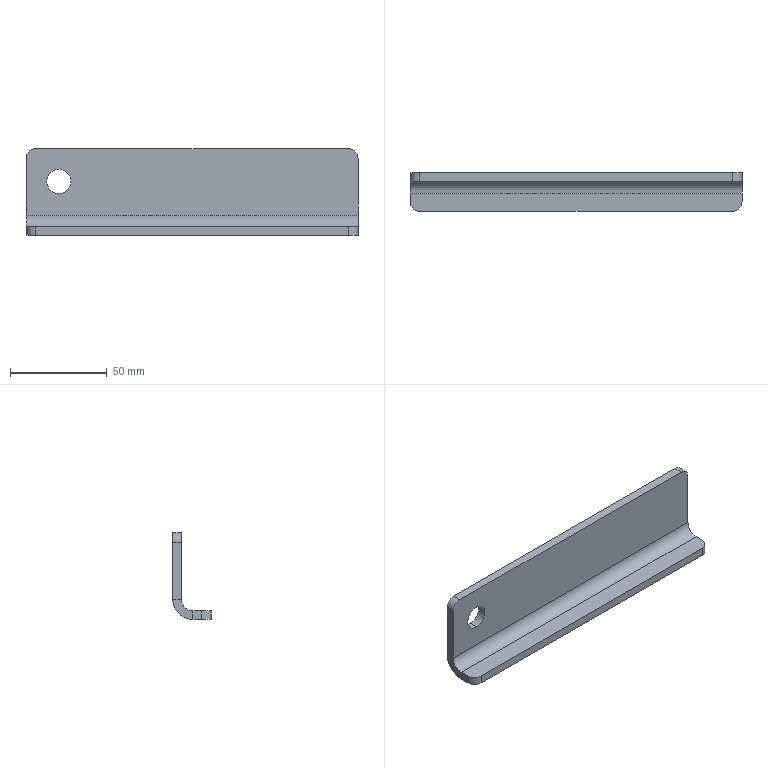Part | SolidWorks | features Fillet 1, FlatPattern 1, ICE 1, SMBaseFlange 1, SheetMetal 1 | 1 solid | 20 faces | box 172 x 20 x 45 mm | volume 43438 mm3 | plane 12 | cylinder 8 | commonest cylinder face diameters 10 x4 12.5 x2 12 x1 21 x1
STEP:
#1=CARTESIAN_POINT('',(17.,15.5,21.75));
#2=VERTEX_POINT('',#1);
#3=CARTESIAN_POINT('',(17.,15.5,34.25));
#4=VERTEX_POINT('',#3);
#5=CARTESIAN_POINT('',(17.,15.5,28.));
#6=DIRECTION('',(0.,1.,0.));
#7=DIRECTION('',(0.,0.,-1.));
#8=AXIS2_PLACEMENT_3D('',#5,#6,#7);
#9=CIRCLE('',#8,6.25);
#10=EDGE_CURVE('',#2,#4,#9,.T.);
#11=ORIENTED_EDGE('',*,*,#10,.F.);
#12=CARTESIAN_POINT('',(17.,20.,21.75));
#13=VERTEX_POINT('',#12);
#14=CARTESIAN_POINT('',(17.,-0.001,21.75));
#15=DIRECTION('',(0.,1.,0.));
#16=VECTOR('',#15,1000.);
#17=LINE('',#14,#16);
#18=EDGE_CURVE('',#2,#13,#17,.T.);
#19=ORIENTED_EDGE('',*,*,#18,.T.);
#20=CARTESIAN_POINT('',(17.,20.,34.25));
#21=VERTEX_POINT('',#20);
#22=CARTESIAN_POINT('',(17.,20.,28.));
#23=DIRECTION('',(0.,1.,0.));
#24=DIRECTION('',(0.,0.,1.));
#25=AXIS2_PLACEMENT_3D('',#22,#23,#24);
#26=CIRCLE('',#25,6.25);
#27=EDGE_CURVE('',#13,#21,#26,.T.);
#28=ORIENTED_EDGE('',*,*,#27,.T.);
#29=CARTESIAN_POINT('',(17.,-0.001,34.25));
#30=DIRECTION('',(0.,1.,0.));
#31=VECTOR('',#30,1000.);
#32=LINE('',#29,#31);
#33=EDGE_CURVE('',#4,#21,#32,.T.);
#34=ORIENTED_EDGE('',*,*,#33,.F.);
#35=EDGE_LOOP('',(#11,#19,#28,#34));
#36=FACE_OUTER_BOUND('',#35,.T.);
#37=CARTESIAN_POINT('',(17.,-0.001,28.));
#38=DIRECTION('',(0.,1.,0.));
#39=DIRECTION('',(0.,0.,1.));
#40=AXIS2_PLACEMENT_3D('',#37,#38,#39);
#41=CYLINDRICAL_SURFACE('',#40,6.25);
#42=ADVANCED_FACE('',(#36),#41,.F.);
#43=CARTESIAN_POINT('',(172.,9.5,0.));
#44=VERTEX_POINT('',#43);
#45=CARTESIAN_POINT('',(172.,9.5,4.5));
#46=VERTEX_POINT('',#45);
#47=CARTESIAN_POINT('',(172.,9.5,0.));
#48=DIRECTION('',(0.,0.,1.));
#49=VECTOR('',#48,1000.);
#50=LINE('',#47,#49);
#51=EDGE_CURVE('',#44,#46,#50,.T.);
#52=ORIENTED_EDGE('',*,*,#51,.F.);
#53=CARTESIAN_POINT('',(172.,20.,10.5));
#54=VERTEX_POINT('',#53);
#55=CARTESIAN_POINT('',(172.,9.5,10.5));
#56=DIRECTION('',(1.,0.,0.));
#57=DIRECTION('',(0.,0.,1.));
#58=AXIS2_PLACEMENT_3D('',#55,#56,#57);
#59=CIRCLE('',#58,10.5);
#60=EDGE_CURVE('',#44,#54,#59,.T.);
#61=ORIENTED_EDGE('',*,*,#60,.T.);
#62=CARTESIAN_POINT('',(172.,15.5,10.5));
#63=VERTEX_POINT('',#62);
#64=CARTESIAN_POINT('',(172.,15.5,10.5));
#65=DIRECTION('',(0.,1.,0.));
#66=VECTOR('',#65,1000.);
#67=LINE('',#64,#66);
#68=EDGE_CURVE('',#63,#54,#67,.T.);
#69=ORIENTED_EDGE('',*,*,#68,.F.);
#70=CARTESIAN_POINT('',(172.,9.5,10.5));
#71=DIRECTION('',(1.,0.,0.));
#72=DIRECTION('',(0.,0.,-1.));
#73=AXIS2_PLACEMENT_3D('',#70,#71,#72);
#74=CIRCLE('',#73,6.);
#75=EDGE_CURVE('',#46,#63,#74,.T.);
#76=ORIENTED_EDGE('',*,*,#75,.F.);
#77=EDGE_LOOP('',(#52,#61,#69,#76));
#78=FACE_OUTER_BOUND('',#77,.T.);
#79=CARTESIAN_POINT('',(172.,9.5,0.));
#80=DIRECTION('',(1.,0.,0.));
#81=DIRECTION('',(0.,0.,-1.));
#82=AXIS2_PLACEMENT_3D('',#79,#80,#81);
#83=PLANE('',#82);
#84=ADVANCED_FACE('',(#78),#83,.T.);
#85=CARTESIAN_POINT('',(172.,5.,4.5));
#86=VERTEX_POINT('',#85);
#87=CARTESIAN_POINT('',(172.,0.,4.5));
#88=DIRECTION('',(0.,1.,0.));
#89=VECTOR('',#88,1000.);
#90=LINE('',#87,#89);
#91=EDGE_CURVE('',#86,#46,#90,.T.);
#92=ORIENTED_EDGE('',*,*,#91,.F.);
#93=CARTESIAN_POINT('',(172.,5.,0.));
#94=VERTEX_POINT('',#93);
#95=CARTESIAN_POINT('',(172.,5.,10.5));
#96=DIRECTION('',(0.,0.,-1.));
#97=VECTOR('',#96,1000.);
#98=LINE('',#95,#97);
#99=EDGE_CURVE('',#86,#94,#98,.T.);
#100=ORIENTED_EDGE('',*,*,#99,.T.);
#101=CARTESIAN_POINT('',(172.,0.,0.));
#102=DIRECTION('',(0.,1.,0.));
#103=VECTOR('',#102,1000.);
#104=LINE('',#101,#103);
#105=EDGE_CURVE('',#94,#44,#104,.T.);
#106=ORIENTED_EDGE('',*,*,#105,.T.);
#107=ORIENTED_EDGE('',*,*,#51,.T.);
#108=EDGE_LOOP('',(#92,#100,#106,#107));
#109=FACE_OUTER_BOUND('',#108,.T.);
#110=CARTESIAN_POINT('',(172.,15.5,10.5));
#111=DIRECTION('',(1.,0.,0.));
#112=DIRECTION('',(0.,0.,-1.));
#113=AXIS2_PLACEMENT_3D('',#110,#111,#112);
#114=PLANE('',#113);
#115=ADVANCED_FACE('',(#109),#114,.T.);
#116=CARTESIAN_POINT('',(0.,20.,10.5));
#117=VERTEX_POINT('',#116);
#118=CARTESIAN_POINT('',(0.,15.5,10.5));
#119=VERTEX_POINT('',#118);
#120=CARTESIAN_POINT('',(0.,20.,10.5));
#121=DIRECTION('',(0.,-1.,0.));
#122=VECTOR('',#121,1000.);
#123=LINE('',#120,#122);
#124=EDGE_CURVE('',#117,#119,#123,.T.);
#125=ORIENTED_EDGE('',*,*,#124,.F.);
#126=CARTESIAN_POINT('',(0.,9.5,0.));
#127=VERTEX_POINT('',#126);
#128=CARTESIAN_POINT('',(0.,9.5,10.5));
#129=DIRECTION('',(1.,0.,0.));
#130=DIRECTION('',(0.,0.,1.));
#131=AXIS2_PLACEMENT_3D('',#128,#129,#130);
#132=CIRCLE('',#131,10.5);
#133=EDGE_CURVE('',#127,#117,#132,.T.);
#134=ORIENTED_EDGE('',*,*,#133,.F.);
#135=CARTESIAN_POINT('',(0.,9.5,4.5));
#136=VERTEX_POINT('',#135);
#137=CARTESIAN_POINT('',(0.,9.5,4.5));
#138=DIRECTION('',(0.,0.,-1.));
#139=VECTOR('',#138,1000.);
#140=LINE('',#137,#139);
#141=EDGE_CURVE('',#136,#127,#140,.T.);
#142=ORIENTED_EDGE('',*,*,#141,.F.);
#143=CARTESIAN_POINT('',(0.,9.5,10.5));
#144=DIRECTION('',(1.,0.,0.));
#145=DIRECTION('',(0.,0.,-1.));
#146=AXIS2_PLACEMENT_3D('',#143,#144,#145);
#147=CIRCLE('',#146,6.);
#148=EDGE_CURVE('',#136,#119,#147,.T.);
#149=ORIENTED_EDGE('',*,*,#148,.T.);
#150=EDGE_LOOP('',(#125,#134,#142,#149));
#151=FACE_OUTER_BOUND('',#150,.T.);
#152=CARTESIAN_POINT('',(0.,20.,10.5));
#153=DIRECTION('',(-1.,0.,0.));
#154=DIRECTION('',(0.,0.,1.));
#155=AXIS2_PLACEMENT_3D('',#152,#153,#154);
#156=PLANE('',#155);
#157=ADVANCED_FACE('',(#151),#156,.T.);
#158=CARTESIAN_POINT('',(0.,15.5,40.));
#159=VERTEX_POINT('',#158);
#160=CARTESIAN_POINT('',(0.,15.5,0.));
#161=DIRECTION('',(0.,0.,1.));
#162=VECTOR('',#161,1000.);
#163=LINE('',#160,#162);
#164=EDGE_CURVE('',#119,#159,#163,.T.);
#165=ORIENTED_EDGE('',*,*,#164,.T.);
#166=CARTESIAN_POINT('',(0.,20.,40.));
#167=VERTEX_POINT('',#166);
#168=CARTESIAN_POINT('',(0.,9.5,40.));
#169=DIRECTION('',(0.,1.,0.));
#170=VECTOR('',#169,1000.);
#171=LINE('',#168,#170);
#172=EDGE_CURVE('',#159,#167,#171,.T.);
#173=ORIENTED_EDGE('',*,*,#172,.T.);
#174=CARTESIAN_POINT('',(0.,20.,0.));
#175=DIRECTION('',(0.,0.,1.));
#176=VECTOR('',#175,1000.);
#177=LINE('',#174,#176);
#178=EDGE_CURVE('',#117,#167,#177,.T.);
#179=ORIENTED_EDGE('',*,*,#178,.F.);
#180=ORIENTED_EDGE('',*,*,#124,.T.);
#181=EDGE_LOOP('',(#165,#173,#179,#180));
#182=FACE_OUTER_BOUND('',#181,.T.);
#183=CARTESIAN_POINT('',(0.,9.5,4.5));
#184=DIRECTION('',(-1.,0.,0.));
#185=DIRECTION('',(0.,0.,1.));
#186=AXIS2_PLACEMENT_3D('',#183,#184,#185);
#187=PLANE('',#186);
#188=ADVANCED_FACE('',(#182),#187,.T.);
#189=CARTESIAN_POINT('',(17.,20.,28.));
#190=DIRECTION('',(0.,1.,0.));
#191=DIRECTION('',(0.,0.,1.));
#192=AXIS2_PLACEMENT_3D('',#189,#190,#191);
#193=CIRCLE('',#192,6.25);
#194=EDGE_CURVE('',#21,#13,#193,.T.);
#195=ORIENTED_EDGE('',*,*,#194,.F.);
#196=ORIENTED_EDGE('',*,*,#27,.F.);
#197=EDGE_LOOP('',(#195,#196));
#198=FACE_BOUND('',#197,.T.);
#199=CARTESIAN_POINT('',(167.,20.,45.));
#200=VERTEX_POINT('',#199);
#201=CARTESIAN_POINT('',(5.,20.,45.));
#202=VERTEX_POINT('',#201);
#203=CARTESIAN_POINT('',(172.,20.,45.));
#204=DIRECTION('',(-1.,0.,0.));
#205=VECTOR('',#204,1000.);
#206=LINE('',#203,#205);
#207=EDGE_CURVE('',#200,#202,#206,.T.);
#208=ORIENTED_EDGE('',*,*,#207,.F.);
#209=CARTESIAN_POINT('',(172.,20.,40.));
#210=VERTEX_POINT('',#209);
#211=CARTESIAN_POINT('',(167.,20.,40.));
#212=DIRECTION('',(0.,1.,0.));
#213=DIRECTION('',(0.,0.,-1.));
#214=AXIS2_PLACEMENT_3D('',#211,#212,#213);
#215=CIRCLE('',#214,5.);
#216=EDGE_CURVE('',#200,#210,#215,.T.);
#217=ORIENTED_EDGE('',*,*,#216,.T.);
#218=CARTESIAN_POINT('',(172.,20.,0.));
#219=DIRECTION('',(0.,0.,1.));
#220=VECTOR('',#219,1000.);
#221=LINE('',#218,#220);
#222=EDGE_CURVE('',#54,#210,#221,.T.);
#223=ORIENTED_EDGE('',*,*,#222,.F.);
#224=CARTESIAN_POINT('',(172.,20.,10.5));
#225=DIRECTION('',(-1.,0.,0.));
#226=VECTOR('',#225,1000.);
#227=LINE('',#224,#226);
#228=EDGE_CURVE('',#54,#117,#227,.T.);
#229=ORIENTED_EDGE('',*,*,#228,.T.);
#230=ORIENTED_EDGE('',*,*,#178,.T.);
#231=CARTESIAN_POINT('',(5.,20.,40.));
#232=DIRECTION('',(0.,1.,0.));
#233=DIRECTION('',(0.,0.,-1.));
#234=AXIS2_PLACEMENT_3D('',#231,#232,#233);
#235=CIRCLE('',#234,5.);
#236=EDGE_CURVE('',#167,#202,#235,.T.);
#237=ORIENTED_EDGE('',*,*,#236,.T.);
#238=EDGE_LOOP('',(#208,#217,#223,#229,#230,#237));
#239=FACE_OUTER_BOUND('',#238,.T.);
#240=CARTESIAN_POINT('',(172.,20.,0.));
#241=DIRECTION('',(0.,-1.,0.));
#242=DIRECTION('',(0.,0.,-1.));
#243=AXIS2_PLACEMENT_3D('',#240,#241,#242);
#244=PLANE('',#243);
#245=ADVANCED_FACE('',(#198,#239),#244,.F.);
#246=CARTESIAN_POINT('',(167.,15.5,45.));
#247=VERTEX_POINT('',#246);
#248=CARTESIAN_POINT('',(5.,15.5,45.));
#249=VERTEX_POINT('',#248);
#250=CARTESIAN_POINT('',(172.,15.5,45.));
#251=DIRECTION('',(-1.,0.,0.));
#252=VECTOR('',#251,1000.);
#253=LINE('',#250,#252);
#254=EDGE_CURVE('',#247,#249,#253,.T.);
#255=ORIENTED_EDGE('',*,*,#254,.F.);
#256=CARTESIAN_POINT('',(167.,15.5,45.));
#257=DIRECTION('',(0.,1.,0.));
#258=VECTOR('',#257,1000.);
#259=LINE('',#256,#258);
#260=EDGE_CURVE('',#247,#200,#259,.T.);
#261=ORIENTED_EDGE('',*,*,#260,.T.);
#262=ORIENTED_EDGE('',*,*,#207,.T.);
#263=CARTESIAN_POINT('',(5.,15.5,45.));
#264=DIRECTION('',(0.,-1.,0.));
#265=VECTOR('',#264,1000.);
#266=LINE('',#263,#265);
#267=EDGE_CURVE('',#202,#249,#266,.T.);
#268=ORIENTED_EDGE('',*,*,#267,.T.);
#269=EDGE_LOOP('',(#255,#261,#262,#268));
#270=FACE_OUTER_BOUND('',#269,.T.);
#271=CARTESIAN_POINT('',(172.,15.5,45.));
#272=DIRECTION('',(0.,0.,1.));
#273=DIRECTION('',(1.,0.,0.));
#274=AXIS2_PLACEMENT_3D('',#271,#272,#273);
#275=PLANE('',#274);
#276=ADVANCED_FACE('',(#270),#275,.T.);
#277=CARTESIAN_POINT('',(17.,15.5,28.));
#278=DIRECTION('',(0.,1.,0.));
#279=DIRECTION('',(0.,0.,-1.));
#280=AXIS2_PLACEMENT_3D('',#277,#278,#279);
#281=CIRCLE('',#280,6.25);
#282=EDGE_CURVE('',#4,#2,#281,.T.);
#283=ORIENTED_EDGE('',*,*,#282,.T.);
#284=ORIENTED_EDGE('',*,*,#10,.T.);
#285=EDGE_LOOP('',(#283,#284));
#286=FACE_BOUND('',#285,.T.);
#287=CARTESIAN_POINT('',(172.,15.5,40.));
#288=VERTEX_POINT('',#287);
#289=CARTESIAN_POINT('',(172.,15.5,0.));
#290=DIRECTION('',(0.,0.,1.));
#291=VECTOR('',#290,1000.);
#292=LINE('',#289,#291);
#293=EDGE_CURVE('',#63,#288,#292,.T.);
#294=ORIENTED_EDGE('',*,*,#293,.T.);
#295=CARTESIAN_POINT('',(167.,15.5,40.));
#296=DIRECTION('',(0.,-1.,0.));
#297=DIRECTION('',(0.,0.,-1.));
#298=AXIS2_PLACEMENT_3D('',#295,#296,#297);
#299=CIRCLE('',#298,5.);
#300=EDGE_CURVE('',#288,#247,#299,.T.);
#301=ORIENTED_EDGE('',*,*,#300,.T.);
#302=ORIENTED_EDGE('',*,*,#254,.T.);
#303=CARTESIAN_POINT('',(5.,15.5,40.));
#304=DIRECTION('',(0.,-1.,0.));
#305=DIRECTION('',(0.,0.,-1.));
#306=AXIS2_PLACEMENT_3D('',#303,#304,#305);
#307=CIRCLE('',#306,5.);
#308=EDGE_CURVE('',#249,#159,#307,.T.);
#309=ORIENTED_EDGE('',*,*,#308,.T.);
#310=ORIENTED_EDGE('',*,*,#164,.F.);
#311=CARTESIAN_POINT('',(172.,15.5,10.5));
#312=DIRECTION('',(-1.,0.,0.));
#313=VECTOR('',#312,1000.);
#314=LINE('',#311,#313);
#315=EDGE_CURVE('',#63,#119,#314,.T.);
#316=ORIENTED_EDGE('',*,*,#315,.F.);
#317=EDGE_LOOP('',(#294,#301,#302,#309,#310,#316));
#318=FACE_OUTER_BOUND('',#317,.T.);
#319=CARTESIAN_POINT('',(172.,15.5,0.));
#320=DIRECTION('',(0.,-1.,0.));
#321=DIRECTION('',(0.,0.,-1.));
#322=AXIS2_PLACEMENT_3D('',#319,#320,#321);
#323=PLANE('',#322);
#324=ADVANCED_FACE('',(#286,#318),#323,.T.);
#325=ORIENTED_EDGE('',*,*,#148,.F.);
#326=CARTESIAN_POINT('',(172.,9.5,4.5));
#327=DIRECTION('',(-1.,0.,0.));
#328=VECTOR('',#327,1000.);
#329=LINE('',#326,#328);
#330=EDGE_CURVE('',#46,#136,#329,.T.);
#331=ORIENTED_EDGE('',*,*,#330,.F.);
#332=ORIENTED_EDGE('',*,*,#75,.T.);
#333=ORIENTED_EDGE('',*,*,#315,.T.);
#334=EDGE_LOOP('',(#325,#331,#332,#333));
#335=FACE_OUTER_BOUND('',#334,.T.);
#336=CARTESIAN_POINT('',(172.,9.5,10.5));
#337=DIRECTION('',(-1.,0.,0.));
#338=DIRECTION('',(0.,0.,1.));
#339=AXIS2_PLACEMENT_3D('',#336,#337,#338);
#340=CYLINDRICAL_SURFACE('',#339,6.);
#341=ADVANCED_FACE('',(#335),#340,.F.);
#342=CARTESIAN_POINT('',(167.,0.,4.5));
#343=VERTEX_POINT('',#342);
#344=CARTESIAN_POINT('',(5.,0.,4.5));
#345=VERTEX_POINT('',#344);
#346=CARTESIAN_POINT('',(172.,0.,4.5));
#347=DIRECTION('',(-1.,0.,0.));
#348=VECTOR('',#347,1000.);
#349=LINE('',#346,#348);
#350=EDGE_CURVE('',#343,#345,#349,.T.);
#351=ORIENTED_EDGE('',*,*,#350,.F.);
#352=CARTESIAN_POINT('',(167.,5.,4.5));
#353=DIRECTION('',(0.,0.,1.));
#354=DIRECTION('',(1.,0.,0.));
#355=AXIS2_PLACEMENT_3D('',#352,#353,#354);
#356=CIRCLE('',#355,5.);
#357=EDGE_CURVE('',#343,#86,#356,.T.);
#358=ORIENTED_EDGE('',*,*,#357,.T.);
#359=ORIENTED_EDGE('',*,*,#91,.T.);
#360=ORIENTED_EDGE('',*,*,#330,.T.);
#361=CARTESIAN_POINT('',(0.,5.,4.5));
#362=VERTEX_POINT('',#361);
#363=CARTESIAN_POINT('',(0.,0.,4.5));
#364=DIRECTION('',(0.,1.,0.));
#365=VECTOR('',#364,1000.);
#366=LINE('',#363,#365);
#367=EDGE_CURVE('',#362,#136,#366,.T.);
#368=ORIENTED_EDGE('',*,*,#367,.F.);
#369=CARTESIAN_POINT('',(5.,5.,4.5));
#370=DIRECTION('',(0.,0.,1.));
#371=DIRECTION('',(1.,0.,0.));
#372=AXIS2_PLACEMENT_3D('',#369,#370,#371);
#373=CIRCLE('',#372,5.);
#374=EDGE_CURVE('',#362,#345,#373,.T.);
#375=ORIENTED_EDGE('',*,*,#374,.T.);
#376=EDGE_LOOP('',(#351,#358,#359,#360,#368,#375));
#377=FACE_OUTER_BOUND('',#376,.T.);
#378=CARTESIAN_POINT('',(172.,0.,4.5));
#379=DIRECTION('',(0.,0.,1.));
#380=DIRECTION('',(1.,0.,0.));
#381=AXIS2_PLACEMENT_3D('',#378,#379,#380);
#382=PLANE('',#381);
#383=ADVANCED_FACE('',(#377),#382,.T.);
#384=CARTESIAN_POINT('',(167.,0.,0.));
#385=VERTEX_POINT('',#384);
#386=CARTESIAN_POINT('',(5.,0.,0.));
#387=VERTEX_POINT('',#386);
#388=CARTESIAN_POINT('',(172.,0.,0.));
#389=DIRECTION('',(-1.,0.,0.));
#390=VECTOR('',#389,1000.);
#391=LINE('',#388,#390);
#392=EDGE_CURVE('',#385,#387,#391,.T.);
#393=ORIENTED_EDGE('',*,*,#392,.F.);
#394=CARTESIAN_POINT('',(167.,0.,0.));
#395=DIRECTION('',(0.,0.,1.));
#396=VECTOR('',#395,1000.);
#397=LINE('',#394,#396);
#398=EDGE_CURVE('',#385,#343,#397,.T.);
#399=ORIENTED_EDGE('',*,*,#398,.T.);
#400=ORIENTED_EDGE('',*,*,#350,.T.);
#401=CARTESIAN_POINT('',(5.,0.,0.));
#402=DIRECTION('',(0.,0.,-1.));
#403=VECTOR('',#402,1000.);
#404=LINE('',#401,#403);
#405=EDGE_CURVE('',#345,#387,#404,.T.);
#406=ORIENTED_EDGE('',*,*,#405,.T.);
#407=EDGE_LOOP('',(#393,#399,#400,#406));
#408=FACE_OUTER_BOUND('',#407,.T.);
#409=CARTESIAN_POINT('',(172.,0.,0.));
#410=DIRECTION('',(0.,-1.,0.));
#411=DIRECTION('',(0.,0.,-1.));
#412=AXIS2_PLACEMENT_3D('',#409,#410,#411);
#413=PLANE('',#412);
#414=ADVANCED_FACE('',(#408),#413,.T.);
#415=ORIENTED_EDGE('',*,*,#105,.F.);
#416=CARTESIAN_POINT('',(167.,5.,0.));
#417=DIRECTION('',(0.,0.,-1.));
#418=DIRECTION('',(1.,0.,0.));
#419=AXIS2_PLACEMENT_3D('',#416,#417,#418);
#420=CIRCLE('',#419,5.);
#421=EDGE_CURVE('',#94,#385,#420,.T.);
#422=ORIENTED_EDGE('',*,*,#421,.T.);
#423=ORIENTED_EDGE('',*,*,#392,.T.);
#424=CARTESIAN_POINT('',(0.,5.,0.));
#425=VERTEX_POINT('',#424);
#426=CARTESIAN_POINT('',(5.,5.,0.));
#427=DIRECTION('',(0.,0.,-1.));
#428=DIRECTION('',(1.,0.,0.));
#429=AXIS2_PLACEMENT_3D('',#426,#427,#428);
#430=CIRCLE('',#429,5.);
#431=EDGE_CURVE('',#387,#425,#430,.T.);
#432=ORIENTED_EDGE('',*,*,#431,.T.);
#433=CARTESIAN_POINT('',(0.,0.,0.));
#434=DIRECTION('',(0.,1.,0.));
#435=VECTOR('',#434,1000.);
#436=LINE('',#433,#435);
#437=EDGE_CURVE('',#425,#127,#436,.T.);
#438=ORIENTED_EDGE('',*,*,#437,.T.);
#439=CARTESIAN_POINT('',(172.,9.5,0.));
#440=DIRECTION('',(-1.,0.,0.));
#441=VECTOR('',#440,1000.);
#442=LINE('',#439,#441);
#443=EDGE_CURVE('',#44,#127,#442,.T.);
#444=ORIENTED_EDGE('',*,*,#443,.F.);
#445=EDGE_LOOP('',(#415,#422,#423,#432,#438,#444));
#446=FACE_OUTER_BOUND('',#445,.T.);
#447=CARTESIAN_POINT('',(172.,0.,0.));
#448=DIRECTION('',(0.,0.,1.));
#449=DIRECTION('',(1.,0.,0.));
#450=AXIS2_PLACEMENT_3D('',#447,#448,#449);
#451=PLANE('',#450);
#452=ADVANCED_FACE('',(#446),#451,.F.);
#453=ORIENTED_EDGE('',*,*,#133,.T.);
#454=ORIENTED_EDGE('',*,*,#228,.F.);
#455=ORIENTED_EDGE('',*,*,#60,.F.);
#456=ORIENTED_EDGE('',*,*,#443,.T.);
#457=EDGE_LOOP('',(#453,#454,#455,#456));
#458=FACE_OUTER_BOUND('',#457,.T.);
#459=CARTESIAN_POINT('',(172.,9.5,10.5));
#460=DIRECTION('',(-1.,0.,0.));
#461=DIRECTION('',(0.,0.,1.));
#462=AXIS2_PLACEMENT_3D('',#459,#460,#461);
#463=CYLINDRICAL_SURFACE('',#462,10.5);
#464=ADVANCED_FACE('',(#458),#463,.T.);
#465=ORIENTED_EDGE('',*,*,#222,.T.);
#466=CARTESIAN_POINT('',(172.,9.5,40.));
#467=DIRECTION('',(0.,-1.,0.));
#468=VECTOR('',#467,1000.);
#469=LINE('',#466,#468);
#470=EDGE_CURVE('',#210,#288,#469,.T.);
#471=ORIENTED_EDGE('',*,*,#470,.T.);
#472=ORIENTED_EDGE('',*,*,#293,.F.);
#473=ORIENTED_EDGE('',*,*,#68,.T.);
#474=EDGE_LOOP('',(#465,#471,#472,#473));
#475=FACE_OUTER_BOUND('',#474,.T.);
#476=CARTESIAN_POINT('',(172.,9.5,10.5));
#477=DIRECTION('',(1.,0.,0.));
#478=DIRECTION('',(0.,0.,-1.));
#479=AXIS2_PLACEMENT_3D('',#476,#477,#478);
#480=PLANE('',#479);
#481=ADVANCED_FACE('',(#475),#480,.T.);
#482=ORIENTED_EDGE('',*,*,#437,.F.);
#483=CARTESIAN_POINT('',(0.,5.,4.5));
#484=DIRECTION('',(0.,0.,1.));
#485=VECTOR('',#484,1000.);
#486=LINE('',#483,#485);
#487=EDGE_CURVE('',#425,#362,#486,.T.);
#488=ORIENTED_EDGE('',*,*,#487,.T.);
#489=ORIENTED_EDGE('',*,*,#367,.T.);
#490=ORIENTED_EDGE('',*,*,#141,.T.);
#491=EDGE_LOOP('',(#482,#488,#489,#490));
#492=FACE_OUTER_BOUND('',#491,.T.);
#493=CARTESIAN_POINT('',(0.,9.5,10.5));
#494=DIRECTION('',(1.,0.,0.));
#495=DIRECTION('',(0.,0.,-1.));
#496=AXIS2_PLACEMENT_3D('',#493,#494,#495);
#497=PLANE('',#496);
#498=ADVANCED_FACE('',(#492),#497,.F.);
#499=ORIENTED_EDGE('',*,*,#18,.F.);
#500=ORIENTED_EDGE('',*,*,#282,.F.);
#501=ORIENTED_EDGE('',*,*,#33,.T.);
#502=ORIENTED_EDGE('',*,*,#194,.T.);
#503=EDGE_LOOP('',(#499,#500,#501,#502));
#504=FACE_OUTER_BOUND('',#503,.T.);
#505=CARTESIAN_POINT('',(17.,-0.001,28.));
#506=DIRECTION('',(0.,1.,0.));
#507=DIRECTION('',(0.,0.,1.));
#508=AXIS2_PLACEMENT_3D('',#505,#506,#507);
#509=CYLINDRICAL_SURFACE('',#508,6.25);
#510=ADVANCED_FACE('',(#504),#509,.F.);
#511=ORIENTED_EDGE('',*,*,#421,.F.);
#512=ORIENTED_EDGE('',*,*,#99,.F.);
#513=ORIENTED_EDGE('',*,*,#357,.F.);
#514=ORIENTED_EDGE('',*,*,#398,.F.);
#515=EDGE_LOOP('',(#511,#512,#513,#514));
#516=FACE_OUTER_BOUND('',#515,.T.);
#517=CARTESIAN_POINT('',(167.,5.,0.));
#518=DIRECTION('',(0.,0.,1.));
#519=DIRECTION('',(1.,0.,0.));
#520=AXIS2_PLACEMENT_3D('',#517,#518,#519);
#521=CYLINDRICAL_SURFACE('',#520,5.);
#522=ADVANCED_FACE('',(#516),#521,.T.);
#523=ORIENTED_EDGE('',*,*,#300,.F.);
#524=ORIENTED_EDGE('',*,*,#470,.F.);
#525=ORIENTED_EDGE('',*,*,#216,.F.);
#526=ORIENTED_EDGE('',*,*,#260,.F.);
#527=EDGE_LOOP('',(#523,#524,#525,#526));
#528=FACE_OUTER_BOUND('',#527,.T.);
#529=CARTESIAN_POINT('',(167.,15.5,40.));
#530=DIRECTION('',(0.,1.,0.));
#531=DIRECTION('',(0.,0.,1.));
#532=AXIS2_PLACEMENT_3D('',#529,#530,#531);
#533=CYLINDRICAL_SURFACE('',#532,5.);
#534=ADVANCED_FACE('',(#528),#533,.T.);
#535=ORIENTED_EDGE('',*,*,#431,.F.);
#536=ORIENTED_EDGE('',*,*,#405,.F.);
#537=ORIENTED_EDGE('',*,*,#374,.F.);
#538=ORIENTED_EDGE('',*,*,#487,.F.);
#539=EDGE_LOOP('',(#535,#536,#537,#538));
#540=FACE_OUTER_BOUND('',#539,.T.);
#541=CARTESIAN_POINT('',(5.,5.,10.5));
#542=DIRECTION('',(0.,0.,-1.));
#543=DIRECTION('',(-1.,0.,0.));
#544=AXIS2_PLACEMENT_3D('',#541,#542,#543);
#545=CYLINDRICAL_SURFACE('',#544,5.);
#546=ADVANCED_FACE('',(#540),#545,.T.);
#547=ORIENTED_EDGE('',*,*,#308,.F.);
#548=ORIENTED_EDGE('',*,*,#267,.F.);
#549=ORIENTED_EDGE('',*,*,#236,.F.);
#550=ORIENTED_EDGE('',*,*,#172,.F.);
#551=EDGE_LOOP('',(#547,#548,#549,#550));
#552=FACE_OUTER_BOUND('',#551,.T.);
#553=CARTESIAN_POINT('',(5.,9.5,40.));
#554=DIRECTION('',(0.,1.,0.));
#555=DIRECTION('',(0.,0.,1.));
#556=AXIS2_PLACEMENT_3D('',#553,#554,#555);
#557=CYLINDRICAL_SURFACE('',#556,5.);
#558=ADVANCED_FACE('',(#552),#557,.T.);
#559=CLOSED_SHELL('',(#42,#84,#115,#157,#188,#245,#276,#324,#341,#383,#414,#452,#464,#481,#498,#510,#522,#534,#546,#558));
#560=MANIFOLD_SOLID_BREP('',#559);
#561=CARTESIAN_POINT('',(0.,0.,0.));
#562=DIRECTION('',(0.,0.,1.));
#563=DIRECTION('',(1.,0.,0.));
#564=AXIS2_PLACEMENT_3D('',#561,#562,#563);
#565=(LENGTH_UNIT()NAMED_UNIT(*)SI_UNIT(.MILLI.,.METRE.));
#566=UNCERTAINTY_MEASURE_WITH_UNIT(LENGTH_MEASURE(0.00001),#565,'','');
#567=(NAMED_UNIT(*)PLANE_ANGLE_UNIT()SI_UNIT($,.RADIAN.));
#568=(NAMED_UNIT(*)SI_UNIT($,.STERADIAN.)SOLID_ANGLE_UNIT());
#569=(GEOMETRIC_REPRESENTATION_CONTEXT(3)GLOBAL_UNCERTAINTY_ASSIGNED_CONTEXT((#566))GLOBAL_UNIT_ASSIGNED_CONTEXT((#565,#567,#568))REPRESENTATION_CONTEXT('',''));
#570=ADVANCED_BREP_SHAPE_REPRESENTATION('',(#560,#564),#569);